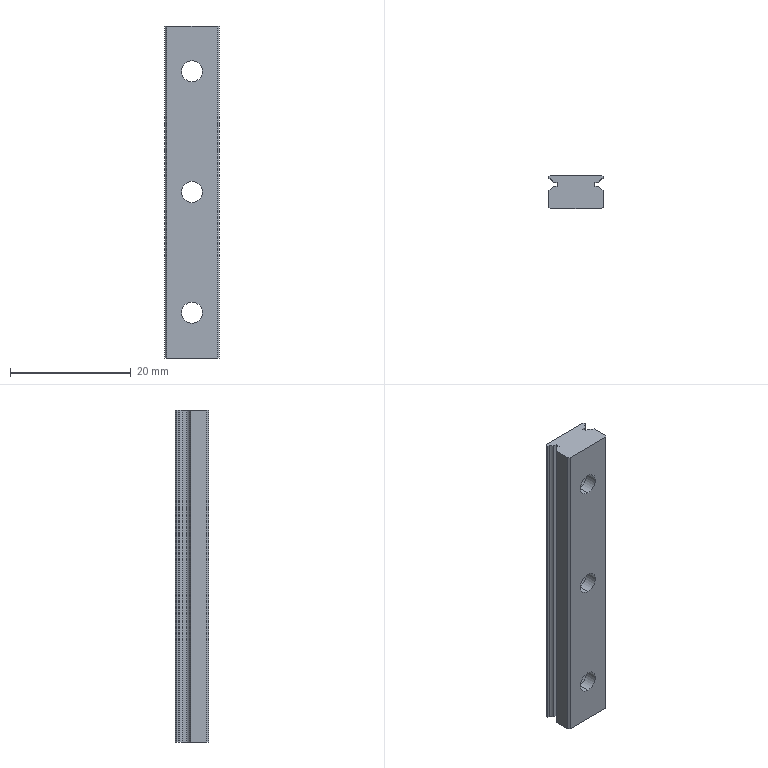Part | SolidWorks | features BaseBody 1 | 1 solid | 41 faces | box 9 x 5.5 x 55 mm | volume 2182 mm3 | plane 25 | cylinder 16 | commonest cylinder face diameters 3.5 x6 6 x6 2.2 x4
STEP:
#1=CARTESIAN_POINT('',(0.,0.,1.75));
#2=VERTEX_POINT('',#1);
#3=CARTESIAN_POINT('',(0.,0.,-1.75));
#4=VERTEX_POINT('',#3);
#5=CARTESIAN_POINT('',(0.,0.,0.));
#6=DIRECTION('',(0.,-1.,0.));
#7=DIRECTION('',(0.,0.,1.));
#8=AXIS2_PLACEMENT_3D('',#5,#6,#7);
#9=CIRCLE('',#8,1.75);
#10=EDGE_CURVE('',#2,#4,#9,.T.);
#11=ORIENTED_EDGE('',*,*,#10,.T.);
#12=CARTESIAN_POINT('',(0.,2.,-1.75));
#13=VERTEX_POINT('',#12);
#14=CARTESIAN_POINT('',(0.,0.,-1.75));
#15=DIRECTION('',(0.,1.,0.));
#16=VECTOR('',#15,1000.);
#17=LINE('',#14,#16);
#18=EDGE_CURVE('',#4,#13,#17,.T.);
#19=ORIENTED_EDGE('',*,*,#18,.T.);
#20=CARTESIAN_POINT('',(0.,2.,1.75));
#21=VERTEX_POINT('',#20);
#22=CARTESIAN_POINT('',(0.,2.,0.));
#23=DIRECTION('',(0.,-1.,0.));
#24=DIRECTION('',(0.,0.,1.));
#25=AXIS2_PLACEMENT_3D('',#22,#23,#24);
#26=CIRCLE('',#25,1.75);
#27=EDGE_CURVE('',#21,#13,#26,.T.);
#28=ORIENTED_EDGE('',*,*,#27,.F.);
#29=CARTESIAN_POINT('',(0.,0.,1.75));
#30=DIRECTION('',(0.,1.,0.));
#31=VECTOR('',#30,1000.);
#32=LINE('',#29,#31);
#33=EDGE_CURVE('',#2,#21,#32,.T.);
#34=ORIENTED_EDGE('',*,*,#33,.F.);
#35=EDGE_LOOP('',(#11,#19,#28,#34));
#36=FACE_OUTER_BOUND('',#35,.T.);
#37=CARTESIAN_POINT('',(0.,0.,0.));
#38=DIRECTION('',(0.,1.,0.));
#39=DIRECTION('',(0.,0.,1.));
#40=AXIS2_PLACEMENT_3D('',#37,#38,#39);
#41=CYLINDRICAL_SURFACE('',#40,1.75);
#42=ADVANCED_FACE('',(#36),#41,.F.);
#43=CARTESIAN_POINT('',(0.,0.,21.75));
#44=VERTEX_POINT('',#43);
#45=CARTESIAN_POINT('',(0.,0.,18.25));
#46=VERTEX_POINT('',#45);
#47=CARTESIAN_POINT('',(0.,0.,20.));
#48=DIRECTION('',(0.,-1.,0.));
#49=DIRECTION('',(0.,0.,1.));
#50=AXIS2_PLACEMENT_3D('',#47,#48,#49);
#51=CIRCLE('',#50,1.75);
#52=EDGE_CURVE('',#44,#46,#51,.T.);
#53=ORIENTED_EDGE('',*,*,#52,.T.);
#54=CARTESIAN_POINT('',(0.,2.,18.25));
#55=VERTEX_POINT('',#54);
#56=CARTESIAN_POINT('',(0.,0.,18.25));
#57=DIRECTION('',(0.,1.,0.));
#58=VECTOR('',#57,1000.);
#59=LINE('',#56,#58);
#60=EDGE_CURVE('',#46,#55,#59,.T.);
#61=ORIENTED_EDGE('',*,*,#60,.T.);
#62=CARTESIAN_POINT('',(0.,2.,21.75));
#63=VERTEX_POINT('',#62);
#64=CARTESIAN_POINT('',(0.,2.,20.));
#65=DIRECTION('',(0.,-1.,0.));
#66=DIRECTION('',(0.,0.,1.));
#67=AXIS2_PLACEMENT_3D('',#64,#65,#66);
#68=CIRCLE('',#67,1.75);
#69=EDGE_CURVE('',#63,#55,#68,.T.);
#70=ORIENTED_EDGE('',*,*,#69,.F.);
#71=CARTESIAN_POINT('',(0.,0.,21.75));
#72=DIRECTION('',(0.,1.,0.));
#73=VECTOR('',#72,1000.);
#74=LINE('',#71,#73);
#75=EDGE_CURVE('',#44,#63,#74,.T.);
#76=ORIENTED_EDGE('',*,*,#75,.F.);
#77=EDGE_LOOP('',(#53,#61,#70,#76));
#78=FACE_OUTER_BOUND('',#77,.T.);
#79=CARTESIAN_POINT('',(0.,0.,20.));
#80=DIRECTION('',(0.,1.,0.));
#81=DIRECTION('',(0.,0.,1.));
#82=AXIS2_PLACEMENT_3D('',#79,#80,#81);
#83=CYLINDRICAL_SURFACE('',#82,1.75);
#84=ADVANCED_FACE('',(#78),#83,.F.);
#85=CARTESIAN_POINT('',(0.,0.,-18.25));
#86=VERTEX_POINT('',#85);
#87=CARTESIAN_POINT('',(0.,0.,-21.75));
#88=VERTEX_POINT('',#87);
#89=CARTESIAN_POINT('',(0.,0.,-20.));
#90=DIRECTION('',(0.,-1.,0.));
#91=DIRECTION('',(0.,0.,1.));
#92=AXIS2_PLACEMENT_3D('',#89,#90,#91);
#93=CIRCLE('',#92,1.75);
#94=EDGE_CURVE('',#86,#88,#93,.T.);
#95=ORIENTED_EDGE('',*,*,#94,.T.);
#96=CARTESIAN_POINT('',(0.,2.,-21.75));
#97=VERTEX_POINT('',#96);
#98=CARTESIAN_POINT('',(0.,0.,-21.75));
#99=DIRECTION('',(0.,1.,0.));
#100=VECTOR('',#99,1000.);
#101=LINE('',#98,#100);
#102=EDGE_CURVE('',#88,#97,#101,.T.);
#103=ORIENTED_EDGE('',*,*,#102,.T.);
#104=CARTESIAN_POINT('',(0.,2.,-18.25));
#105=VERTEX_POINT('',#104);
#106=CARTESIAN_POINT('',(0.,2.,-20.));
#107=DIRECTION('',(0.,-1.,0.));
#108=DIRECTION('',(0.,0.,1.));
#109=AXIS2_PLACEMENT_3D('',#106,#107,#108);
#110=CIRCLE('',#109,1.75);
#111=EDGE_CURVE('',#105,#97,#110,.T.);
#112=ORIENTED_EDGE('',*,*,#111,.F.);
#113=CARTESIAN_POINT('',(0.,0.,-18.25));
#114=DIRECTION('',(0.,1.,0.));
#115=VECTOR('',#114,1000.);
#116=LINE('',#113,#115);
#117=EDGE_CURVE('',#86,#105,#116,.T.);
#118=ORIENTED_EDGE('',*,*,#117,.F.);
#119=EDGE_LOOP('',(#95,#103,#112,#118));
#120=FACE_OUTER_BOUND('',#119,.T.);
#121=CARTESIAN_POINT('',(0.,0.,-20.));
#122=DIRECTION('',(0.,1.,0.));
#123=DIRECTION('',(0.,0.,1.));
#124=AXIS2_PLACEMENT_3D('',#121,#122,#123);
#125=CYLINDRICAL_SURFACE('',#124,1.75);
#126=ADVANCED_FACE('',(#120),#125,.F.);
#127=CARTESIAN_POINT('',(0.,2.,-3.));
#128=VERTEX_POINT('',#127);
#129=CARTESIAN_POINT('',(0.,2.,3.));
#130=VERTEX_POINT('',#129);
#131=CARTESIAN_POINT('',(0.,2.,0.));
#132=DIRECTION('',(0.,1.,0.));
#133=DIRECTION('',(0.,0.,1.));
#134=AXIS2_PLACEMENT_3D('',#131,#132,#133);
#135=CIRCLE('',#134,3.);
#136=EDGE_CURVE('',#128,#130,#135,.T.);
#137=ORIENTED_EDGE('',*,*,#136,.F.);
#138=CARTESIAN_POINT('',(0.,5.5,-3.));
#139=VERTEX_POINT('',#138);
#140=CARTESIAN_POINT('',(0.,0.,-3.));
#141=DIRECTION('',(0.,1.,0.));
#142=VECTOR('',#141,1000.);
#143=LINE('',#140,#142);
#144=EDGE_CURVE('',#128,#139,#143,.T.);
#145=ORIENTED_EDGE('',*,*,#144,.T.);
#146=CARTESIAN_POINT('',(0.,5.5,3.));
#147=VERTEX_POINT('',#146);
#148=CARTESIAN_POINT('',(0.,5.5,0.));
#149=DIRECTION('',(0.,1.,0.));
#150=DIRECTION('',(0.,0.,1.));
#151=AXIS2_PLACEMENT_3D('',#148,#149,#150);
#152=CIRCLE('',#151,3.);
#153=EDGE_CURVE('',#139,#147,#152,.T.);
#154=ORIENTED_EDGE('',*,*,#153,.T.);
#155=CARTESIAN_POINT('',(0.,0.,3.));
#156=DIRECTION('',(0.,1.,0.));
#157=VECTOR('',#156,1000.);
#158=LINE('',#155,#157);
#159=EDGE_CURVE('',#130,#147,#158,.T.);
#160=ORIENTED_EDGE('',*,*,#159,.F.);
#161=EDGE_LOOP('',(#137,#145,#154,#160));
#162=FACE_OUTER_BOUND('',#161,.T.);
#163=CARTESIAN_POINT('',(0.,0.,0.));
#164=DIRECTION('',(0.,1.,0.));
#165=DIRECTION('',(0.,0.,1.));
#166=AXIS2_PLACEMENT_3D('',#163,#164,#165);
#167=CYLINDRICAL_SURFACE('',#166,3.);
#168=ADVANCED_FACE('',(#162),#167,.F.);
#169=CARTESIAN_POINT('',(0.,2.,17.));
#170=VERTEX_POINT('',#169);
#171=CARTESIAN_POINT('',(0.,2.,23.));
#172=VERTEX_POINT('',#171);
#173=CARTESIAN_POINT('',(0.,2.,20.));
#174=DIRECTION('',(0.,1.,0.));
#175=DIRECTION('',(0.,0.,1.));
#176=AXIS2_PLACEMENT_3D('',#173,#174,#175);
#177=CIRCLE('',#176,3.);
#178=EDGE_CURVE('',#170,#172,#177,.T.);
#179=ORIENTED_EDGE('',*,*,#178,.F.);
#180=CARTESIAN_POINT('',(0.,5.5,17.));
#181=VERTEX_POINT('',#180);
#182=CARTESIAN_POINT('',(0.,0.,17.));
#183=DIRECTION('',(0.,1.,0.));
#184=VECTOR('',#183,1000.);
#185=LINE('',#182,#184);
#186=EDGE_CURVE('',#170,#181,#185,.T.);
#187=ORIENTED_EDGE('',*,*,#186,.T.);
#188=CARTESIAN_POINT('',(0.,5.5,23.));
#189=VERTEX_POINT('',#188);
#190=CARTESIAN_POINT('',(0.,5.5,20.));
#191=DIRECTION('',(0.,1.,0.));
#192=DIRECTION('',(0.,0.,1.));
#193=AXIS2_PLACEMENT_3D('',#190,#191,#192);
#194=CIRCLE('',#193,3.);
#195=EDGE_CURVE('',#181,#189,#194,.T.);
#196=ORIENTED_EDGE('',*,*,#195,.T.);
#197=CARTESIAN_POINT('',(0.,0.,23.));
#198=DIRECTION('',(0.,1.,0.));
#199=VECTOR('',#198,1000.);
#200=LINE('',#197,#199);
#201=EDGE_CURVE('',#172,#189,#200,.T.);
#202=ORIENTED_EDGE('',*,*,#201,.F.);
#203=EDGE_LOOP('',(#179,#187,#196,#202));
#204=FACE_OUTER_BOUND('',#203,.T.);
#205=CARTESIAN_POINT('',(0.,0.,20.));
#206=DIRECTION('',(0.,1.,0.));
#207=DIRECTION('',(0.,0.,1.));
#208=AXIS2_PLACEMENT_3D('',#205,#206,#207);
#209=CYLINDRICAL_SURFACE('',#208,3.);
#210=ADVANCED_FACE('',(#204),#209,.F.);
#211=CARTESIAN_POINT('',(0.,2.,-23.));
#212=VERTEX_POINT('',#211);
#213=CARTESIAN_POINT('',(0.,2.,-17.));
#214=VERTEX_POINT('',#213);
#215=CARTESIAN_POINT('',(0.,2.,-20.));
#216=DIRECTION('',(0.,1.,0.));
#217=DIRECTION('',(0.,0.,1.));
#218=AXIS2_PLACEMENT_3D('',#215,#216,#217);
#219=CIRCLE('',#218,3.);
#220=EDGE_CURVE('',#212,#214,#219,.T.);
#221=ORIENTED_EDGE('',*,*,#220,.F.);
#222=CARTESIAN_POINT('',(0.,5.5,-23.));
#223=VERTEX_POINT('',#222);
#224=CARTESIAN_POINT('',(0.,0.,-23.));
#225=DIRECTION('',(0.,1.,0.));
#226=VECTOR('',#225,1000.);
#227=LINE('',#224,#226);
#228=EDGE_CURVE('',#212,#223,#227,.T.);
#229=ORIENTED_EDGE('',*,*,#228,.T.);
#230=CARTESIAN_POINT('',(0.,5.5,-17.));
#231=VERTEX_POINT('',#230);
#232=CARTESIAN_POINT('',(0.,5.5,-20.));
#233=DIRECTION('',(0.,1.,0.));
#234=DIRECTION('',(0.,0.,1.));
#235=AXIS2_PLACEMENT_3D('',#232,#233,#234);
#236=CIRCLE('',#235,3.);
#237=EDGE_CURVE('',#223,#231,#236,.T.);
#238=ORIENTED_EDGE('',*,*,#237,.T.);
#239=CARTESIAN_POINT('',(0.,0.,-17.));
#240=DIRECTION('',(0.,1.,0.));
#241=VECTOR('',#240,1000.);
#242=LINE('',#239,#241);
#243=EDGE_CURVE('',#214,#231,#242,.T.);
#244=ORIENTED_EDGE('',*,*,#243,.F.);
#245=EDGE_LOOP('',(#221,#229,#238,#244));
#246=FACE_OUTER_BOUND('',#245,.T.);
#247=CARTESIAN_POINT('',(0.,0.,-20.));
#248=DIRECTION('',(0.,1.,0.));
#249=DIRECTION('',(0.,0.,1.));
#250=AXIS2_PLACEMENT_3D('',#247,#248,#249);
#251=CYLINDRICAL_SURFACE('',#250,3.);
#252=ADVANCED_FACE('',(#246),#251,.F.);
#253=ORIENTED_EDGE('',*,*,#10,.F.);
#254=CARTESIAN_POINT('',(0.,0.,0.));
#255=DIRECTION('',(0.,-1.,0.));
#256=DIRECTION('',(0.,0.,1.));
#257=AXIS2_PLACEMENT_3D('',#254,#255,#256);
#258=CIRCLE('',#257,1.75);
#259=EDGE_CURVE('',#4,#2,#258,.T.);
#260=ORIENTED_EDGE('',*,*,#259,.F.);
#261=EDGE_LOOP('',(#253,#260));
#262=FACE_BOUND('',#261,.T.);
#263=ORIENTED_EDGE('',*,*,#52,.F.);
#264=CARTESIAN_POINT('',(0.,0.,20.));
#265=DIRECTION('',(0.,-1.,0.));
#266=DIRECTION('',(0.,0.,1.));
#267=AXIS2_PLACEMENT_3D('',#264,#265,#266);
#268=CIRCLE('',#267,1.75);
#269=EDGE_CURVE('',#46,#44,#268,.T.);
#270=ORIENTED_EDGE('',*,*,#269,.F.);
#271=EDGE_LOOP('',(#263,#270));
#272=FACE_BOUND('',#271,.T.);
#273=ORIENTED_EDGE('',*,*,#94,.F.);
#274=CARTESIAN_POINT('',(0.,0.,-20.));
#275=DIRECTION('',(0.,-1.,0.));
#276=DIRECTION('',(0.,0.,1.));
#277=AXIS2_PLACEMENT_3D('',#274,#275,#276);
#278=CIRCLE('',#277,1.75);
#279=EDGE_CURVE('',#88,#86,#278,.T.);
#280=ORIENTED_EDGE('',*,*,#279,.F.);
#281=EDGE_LOOP('',(#273,#280));
#282=FACE_BOUND('',#281,.T.);
#283=CARTESIAN_POINT('',(-4.2,0.,27.5));
#284=VERTEX_POINT('',#283);
#285=CARTESIAN_POINT('',(4.2,0.,27.5));
#286=VERTEX_POINT('',#285);
#287=CARTESIAN_POINT('',(-4.2,0.,27.5));
#288=DIRECTION('',(1.,0.,0.));
#289=VECTOR('',#288,1000.);
#290=LINE('',#287,#289);
#291=EDGE_CURVE('',#284,#286,#290,.T.);
#292=ORIENTED_EDGE('',*,*,#291,.F.);
#293=CARTESIAN_POINT('',(-4.2,0.,-27.5));
#294=VERTEX_POINT('',#293);
#295=CARTESIAN_POINT('',(-4.2,0.,27.5));
#296=DIRECTION('',(0.,0.,1.));
#297=VECTOR('',#296,1000.);
#298=LINE('',#295,#297);
#299=EDGE_CURVE('',#294,#284,#298,.T.);
#300=ORIENTED_EDGE('',*,*,#299,.F.);
#301=CARTESIAN_POINT('',(4.2,0.,-27.5));
#302=VERTEX_POINT('',#301);
#303=CARTESIAN_POINT('',(-4.2,0.,-27.5));
#304=DIRECTION('',(-1.,0.,0.));
#305=VECTOR('',#304,1000.);
#306=LINE('',#303,#305);
#307=EDGE_CURVE('',#302,#294,#306,.T.);
#308=ORIENTED_EDGE('',*,*,#307,.F.);
#309=CARTESIAN_POINT('',(4.2,0.,27.5));
#310=DIRECTION('',(0.,0.,-1.));
#311=VECTOR('',#310,1000.);
#312=LINE('',#309,#311);
#313=EDGE_CURVE('',#286,#302,#312,.T.);
#314=ORIENTED_EDGE('',*,*,#313,.F.);
#315=EDGE_LOOP('',(#292,#300,#308,#314));
#316=FACE_OUTER_BOUND('',#315,.T.);
#317=CARTESIAN_POINT('',(-4.2,0.,27.5));
#318=DIRECTION('',(0.,1.,0.));
#319=DIRECTION('',(0.,0.,1.));
#320=AXIS2_PLACEMENT_3D('',#317,#318,#319);
#321=PLANE('',#320);
#322=ADVANCED_FACE('',(#262,#272,#282,#316),#321,.F.);
#323=ORIENTED_EDGE('',*,*,#18,.F.);
#324=ORIENTED_EDGE('',*,*,#259,.T.);
#325=ORIENTED_EDGE('',*,*,#33,.T.);
#326=CARTESIAN_POINT('',(0.,2.,0.));
#327=DIRECTION('',(0.,-1.,0.));
#328=DIRECTION('',(0.,0.,1.));
#329=AXIS2_PLACEMENT_3D('',#326,#327,#328);
#330=CIRCLE('',#329,1.75);
#331=EDGE_CURVE('',#13,#21,#330,.T.);
#332=ORIENTED_EDGE('',*,*,#331,.F.);
#333=EDGE_LOOP('',(#323,#324,#325,#332));
#334=FACE_OUTER_BOUND('',#333,.T.);
#335=CARTESIAN_POINT('',(0.,0.,0.));
#336=DIRECTION('',(0.,1.,0.));
#337=DIRECTION('',(0.,0.,1.));
#338=AXIS2_PLACEMENT_3D('',#335,#336,#337);
#339=CYLINDRICAL_SURFACE('',#338,1.75);
#340=ADVANCED_FACE('',(#334),#339,.F.);
#341=ORIENTED_EDGE('',*,*,#60,.F.);
#342=ORIENTED_EDGE('',*,*,#269,.T.);
#343=ORIENTED_EDGE('',*,*,#75,.T.);
#344=CARTESIAN_POINT('',(0.,2.,20.));
#345=DIRECTION('',(0.,-1.,0.));
#346=DIRECTION('',(0.,0.,1.));
#347=AXIS2_PLACEMENT_3D('',#344,#345,#346);
#348=CIRCLE('',#347,1.75);
#349=EDGE_CURVE('',#55,#63,#348,.T.);
#350=ORIENTED_EDGE('',*,*,#349,.F.);
#351=EDGE_LOOP('',(#341,#342,#343,#350));
#352=FACE_OUTER_BOUND('',#351,.T.);
#353=CARTESIAN_POINT('',(0.,0.,20.));
#354=DIRECTION('',(0.,1.,0.));
#355=DIRECTION('',(0.,0.,1.));
#356=AXIS2_PLACEMENT_3D('',#353,#354,#355);
#357=CYLINDRICAL_SURFACE('',#356,1.75);
#358=ADVANCED_FACE('',(#352),#357,.F.);
#359=ORIENTED_EDGE('',*,*,#102,.F.);
#360=ORIENTED_EDGE('',*,*,#279,.T.);
#361=ORIENTED_EDGE('',*,*,#117,.T.);
#362=CARTESIAN_POINT('',(0.,2.,-20.));
#363=DIRECTION('',(0.,-1.,0.));
#364=DIRECTION('',(0.,0.,1.));
#365=AXIS2_PLACEMENT_3D('',#362,#363,#364);
#366=CIRCLE('',#365,1.75);
#367=EDGE_CURVE('',#97,#105,#366,.T.);
#368=ORIENTED_EDGE('',*,*,#367,.F.);
#369=EDGE_LOOP('',(#359,#360,#361,#368));
#370=FACE_OUTER_BOUND('',#369,.T.);
#371=CARTESIAN_POINT('',(0.,0.,-20.));
#372=DIRECTION('',(0.,1.,0.));
#373=DIRECTION('',(0.,0.,1.));
#374=AXIS2_PLACEMENT_3D('',#371,#372,#373);
#375=CYLINDRICAL_SURFACE('',#374,1.75);
#376=ADVANCED_FACE('',(#370),#375,.F.);
#377=CARTESIAN_POINT('',(4.5,0.3,27.5));
#378=VERTEX_POINT('',#377);
#379=CARTESIAN_POINT('',(4.2,0.,27.5));
#380=DIRECTION('',(0.7071,0.7071,0.));
#381=VECTOR('',#380,1000.);
#382=LINE('',#379,#381);
#383=EDGE_CURVE('',#286,#378,#382,.T.);
#384=ORIENTED_EDGE('',*,*,#383,.F.);
#385=ORIENTED_EDGE('',*,*,#313,.T.);
#386=CARTESIAN_POINT('',(4.5,0.3,-27.5));
#387=VERTEX_POINT('',#386);
#388=CARTESIAN_POINT('',(4.2,0.,-27.5));
#389=DIRECTION('',(-0.7071,-0.7071,0.));
#390=VECTOR('',#389,1000.);
#391=LINE('',#388,#390);
#392=EDGE_CURVE('',#387,#302,#391,.T.);
#393=ORIENTED_EDGE('',*,*,#392,.F.);
#394=CARTESIAN_POINT('',(4.5,0.3,27.5));
#395=DIRECTION('',(0.,0.,-1.));
#396=VECTOR('',#395,1000.);
#397=LINE('',#394,#396);
#398=EDGE_CURVE('',#378,#387,#397,.T.);
#399=ORIENTED_EDGE('',*,*,#398,.F.);
#400=EDGE_LOOP('',(#384,#385,#393,#399));
#401=FACE_OUTER_BOUND('',#400,.T.);
#402=CARTESIAN_POINT('',(4.2,0.,27.5));
#403=DIRECTION('',(-0.7071,0.7071,0.));
#404=DIRECTION('',(-0.7071,-0.7071,0.));
#405=AXIS2_PLACEMENT_3D('',#402,#403,#404);
#406=PLANE('',#405);
#407=ADVANCED_FACE('',(#401),#406,.F.);
#408=CARTESIAN_POINT('',(4.222,4.883,27.5));
#409=VERTEX_POINT('',#408);
#410=CARTESIAN_POINT('',(4.5,5.043,27.5));
#411=VERTEX_POINT('',#410);
#412=CARTESIAN_POINT('',(4.222,4.883,27.5));
#413=DIRECTION('',(0.8661,0.5,0.));
#414=VECTOR('',#413,1000.);
#415=LINE('',#412,#414);
#416=EDGE_CURVE('',#409,#411,#415,.T.);
#417=ORIENTED_EDGE('',*,*,#416,.T.);
#418=CARTESIAN_POINT('',(4.5,5.3,27.5));
#419=VERTEX_POINT('',#418);
#420=CARTESIAN_POINT('',(4.5,5.043,27.5));
#421=DIRECTION('',(0.,1.,0.));
#422=VECTOR('',#421,1000.);
#423=LINE('',#420,#422);
#424=EDGE_CURVE('',#411,#419,#423,.T.);
#425=ORIENTED_EDGE('',*,*,#424,.T.);
#426=CARTESIAN_POINT('',(4.3,5.5,27.5));
#427=VERTEX_POINT('',#426);
#428=CARTESIAN_POINT('',(4.5,5.3,27.5));
#429=DIRECTION('',(-0.7071,0.7071,0.));
#430=VECTOR('',#429,1000.);
#431=LINE('',#428,#430);
#432=EDGE_CURVE('',#419,#427,#431,.T.);
#433=ORIENTED_EDGE('',*,*,#432,.T.);
#434=CARTESIAN_POINT('',(-4.3,5.5,27.5));
#435=VERTEX_POINT('',#434);
#436=CARTESIAN_POINT('',(-4.771,5.5,27.5));
#437=DIRECTION('',(-1.,0.,0.));
#438=VECTOR('',#437,1000.);
#439=LINE('',#436,#438);
#440=EDGE_CURVE('',#427,#435,#439,.T.);
#441=ORIENTED_EDGE('',*,*,#440,.T.);
#442=CARTESIAN_POINT('',(-4.5,5.3,27.5));
#443=VERTEX_POINT('',#442);
#444=CARTESIAN_POINT('',(-4.3,5.5,27.5));
#445=DIRECTION('',(-0.7071,-0.7071,0.));
#446=VECTOR('',#445,1000.);
#447=LINE('',#444,#446);
#448=EDGE_CURVE('',#435,#443,#447,.T.);
#449=ORIENTED_EDGE('',*,*,#448,.T.);
#450=CARTESIAN_POINT('',(-4.5,5.043,27.5));
#451=VERTEX_POINT('',#450);
#452=CARTESIAN_POINT('',(-4.5,5.3,27.5));
#453=DIRECTION('',(0.,-1.,0.));
#454=VECTOR('',#453,1000.);
#455=LINE('',#452,#454);
#456=EDGE_CURVE('',#443,#451,#455,.T.);
#457=ORIENTED_EDGE('',*,*,#456,.T.);
#458=CARTESIAN_POINT('',(-4.222,4.883,27.5));
#459=VERTEX_POINT('',#458);
#460=CARTESIAN_POINT('',(-4.5,5.043,27.5));
#461=DIRECTION('',(0.8661,-0.5,0.));
#462=VECTOR('',#461,1000.);
#463=LINE('',#460,#462);
#464=EDGE_CURVE('',#451,#459,#463,.T.);
#465=ORIENTED_EDGE('',*,*,#464,.T.);
#466=CARTESIAN_POINT('',(-3.755,4.35,27.5));
#467=VERTEX_POINT('',#466);
#468=CARTESIAN_POINT('',(-4.771,3.93,27.5));
#469=DIRECTION('',(0.,0.,-1.));
#470=DIRECTION('',(1.,0.,0.));
#471=AXIS2_PLACEMENT_3D('',#468,#469,#470);
#472=CIRCLE('',#471,1.1);
#473=EDGE_CURVE('',#459,#467,#472,.T.);
#474=ORIENTED_EDGE('',*,*,#473,.T.);
#475=CARTESIAN_POINT('',(-3.1,4.35,27.5));
#476=VERTEX_POINT('',#475);
#477=CARTESIAN_POINT('',(-3.755,4.35,27.5));
#478=DIRECTION('',(1.,0.,0.));
#479=VECTOR('',#478,1000.);
#480=LINE('',#477,#479);
#481=EDGE_CURVE('',#467,#476,#480,.T.);
#482=ORIENTED_EDGE('',*,*,#481,.T.);
#483=CARTESIAN_POINT('',(-3.1,3.65,27.5));
#484=VERTEX_POINT('',#483);
#485=CARTESIAN_POINT('',(-3.1,4.35,27.5));
#486=DIRECTION('',(0.,-1.,0.));
#487=VECTOR('',#486,1000.);
#488=LINE('',#485,#487);
#489=EDGE_CURVE('',#476,#484,#488,.T.);
#490=ORIENTED_EDGE('',*,*,#489,.T.);
#491=CARTESIAN_POINT('',(-3.755,3.65,27.5));
#492=VERTEX_POINT('',#491);
#493=CARTESIAN_POINT('',(-3.1,3.65,27.5));
#494=DIRECTION('',(-1.,0.,0.));
#495=VECTOR('',#494,1000.);
#496=LINE('',#493,#495);
#497=EDGE_CURVE('',#484,#492,#496,.T.);
#498=ORIENTED_EDGE('',*,*,#497,.T.);
#499=CARTESIAN_POINT('',(-4.222,3.117,27.5));
#500=VERTEX_POINT('',#499);
#501=CARTESIAN_POINT('',(-4.772,4.07,27.5));
#502=DIRECTION('',(0.,0.,-1.));
#503=DIRECTION('',(1.,0.,0.));
#504=AXIS2_PLACEMENT_3D('',#501,#502,#503);
#505=CIRCLE('',#504,1.1);
#506=EDGE_CURVE('',#492,#500,#505,.T.);
#507=ORIENTED_EDGE('',*,*,#506,.T.);
#508=CARTESIAN_POINT('',(-4.5,2.957,27.5));
#509=VERTEX_POINT('',#508);
#510=CARTESIAN_POINT('',(-4.222,3.117,27.5));
#511=DIRECTION('',(-0.8661,-0.5,0.));
#512=VECTOR('',#511,1000.);
#513=LINE('',#510,#512);
#514=EDGE_CURVE('',#500,#509,#513,.T.);
#515=ORIENTED_EDGE('',*,*,#514,.T.);
#516=CARTESIAN_POINT('',(-4.5,0.3,27.5));
#517=VERTEX_POINT('',#516);
#518=CARTESIAN_POINT('',(-4.5,3.93,27.5));
#519=DIRECTION('',(0.,-1.,0.));
#520=VECTOR('',#519,1000.);
#521=LINE('',#518,#520);
#522=EDGE_CURVE('',#509,#517,#521,.T.);
#523=ORIENTED_EDGE('',*,*,#522,.T.);
#524=CARTESIAN_POINT('',(-4.5,0.3,27.5));
#525=DIRECTION('',(0.7071,-0.7071,0.));
#526=VECTOR('',#525,1000.);
#527=LINE('',#524,#526);
#528=EDGE_CURVE('',#517,#284,#527,.T.);
#529=ORIENTED_EDGE('',*,*,#528,.T.);
#530=ORIENTED_EDGE('',*,*,#291,.T.);
#531=ORIENTED_EDGE('',*,*,#383,.T.);
#532=CARTESIAN_POINT('',(4.5,2.957,27.5));
#533=VERTEX_POINT('',#532);
#534=CARTESIAN_POINT('',(4.5,3.93,27.5));
#535=DIRECTION('',(0.,1.,0.));
#536=VECTOR('',#535,1000.);
#537=LINE('',#534,#536);
#538=EDGE_CURVE('',#378,#533,#537,.T.);
#539=ORIENTED_EDGE('',*,*,#538,.T.);
#540=CARTESIAN_POINT('',(4.222,3.117,27.5));
#541=VERTEX_POINT('',#540);
#542=CARTESIAN_POINT('',(4.5,2.957,27.5));
#543=DIRECTION('',(-0.8661,0.5,0.));
#544=VECTOR('',#543,1000.);
#545=LINE('',#542,#544);
#546=EDGE_CURVE('',#533,#541,#545,.T.);
#547=ORIENTED_EDGE('',*,*,#546,.T.);
#548=CARTESIAN_POINT('',(3.755,3.65,27.5));
#549=VERTEX_POINT('',#548);
#550=CARTESIAN_POINT('',(4.772,4.07,27.5));
#551=DIRECTION('',(0.,0.,-1.));
#552=DIRECTION('',(1.,0.,0.));
#553=AXIS2_PLACEMENT_3D('',#550,#551,#552);
#554=CIRCLE('',#553,1.1);
#555=EDGE_CURVE('',#541,#549,#554,.T.);
#556=ORIENTED_EDGE('',*,*,#555,.T.);
#557=CARTESIAN_POINT('',(3.1,3.65,27.5));
#558=VERTEX_POINT('',#557);
#559=CARTESIAN_POINT('',(3.755,3.65,27.5));
#560=DIRECTION('',(-1.,0.,0.));
#561=VECTOR('',#560,1000.);
#562=LINE('',#559,#561);
#563=EDGE_CURVE('',#549,#558,#562,.T.);
#564=ORIENTED_EDGE('',*,*,#563,.T.);
#565=CARTESIAN_POINT('',(3.1,4.35,27.5));
#566=VERTEX_POINT('',#565);
#567=CARTESIAN_POINT('',(3.1,3.65,27.5));
#568=DIRECTION('',(0.,1.,0.));
#569=VECTOR('',#568,1000.);
#570=LINE('',#567,#569);
#571=EDGE_CURVE('',#558,#566,#570,.T.);
#572=ORIENTED_EDGE('',*,*,#571,.T.);
#573=CARTESIAN_POINT('',(3.755,4.35,27.5));
#574=VERTEX_POINT('',#573);
#575=CARTESIAN_POINT('',(3.1,4.35,27.5));
#576=DIRECTION('',(1.,0.,0.));
#577=VECTOR('',#576,1000.);
#578=LINE('',#575,#577);
#579=EDGE_CURVE('',#566,#574,#578,.T.);
#580=ORIENTED_EDGE('',*,*,#579,.T.);
#581=CARTESIAN_POINT('',(4.771,3.93,27.5));
#582=DIRECTION('',(0.,0.,-1.));
#583=DIRECTION('',(1.,0.,0.));
#584=AXIS2_PLACEMENT_3D('',#581,#582,#583);
#585=CIRCLE('',#584,1.1);
#586=EDGE_CURVE('',#574,#409,#585,.T.);
#587=ORIENTED_EDGE('',*,*,#586,.T.);
#588=EDGE_LOOP('',(#417,#425,#433,#441,#449,#457,#465,#474,#482,#490,#498,#507,#515,#523,#529,#530,#531,#539,#547,#556,#564,#572,#580,#587));
#589=FACE_OUTER_BOUND('',#588,.T.);
#590=CARTESIAN_POINT('',(-4.771,3.93,27.5));
#591=DIRECTION('',(0.,0.,1.));
#592=DIRECTION('',(1.,0.,0.));
#593=AXIS2_PLACEMENT_3D('',#590,#591,#592);
#594=PLANE('',#593);
#595=ADVANCED_FACE('',(#589),#594,.T.);
#596=ORIENTED_EDGE('',*,*,#528,.F.);
#597=CARTESIAN_POINT('',(-4.5,0.3,-27.5));
#598=VERTEX_POINT('',#597);
#599=CARTESIAN_POINT('',(-4.5,0.3,27.5));
#600=DIRECTION('',(0.,0.,1.));
#601=VECTOR('',#600,1000.);
#602=LINE('',#599,#601);
#603=EDGE_CURVE('',#598,#517,#602,.T.);
#604=ORIENTED_EDGE('',*,*,#603,.F.);
#605=CARTESIAN_POINT('',(-4.5,0.3,-27.5));
#606=DIRECTION('',(-0.7071,0.7071,0.));
#607=VECTOR('',#606,1000.);
#608=LINE('',#605,#607);
#609=EDGE_CURVE('',#294,#598,#608,.T.);
#610=ORIENTED_EDGE('',*,*,#609,.F.);
#611=ORIENTED_EDGE('',*,*,#299,.T.);
#612=EDGE_LOOP('',(#596,#604,#610,#611));
#613=FACE_OUTER_BOUND('',#612,.T.);
#614=CARTESIAN_POINT('',(-4.5,0.3,27.5));
#615=DIRECTION('',(0.7071,0.7071,0.));
#616=DIRECTION('',(-0.7071,0.7071,0.));
#617=AXIS2_PLACEMENT_3D('',#614,#615,#616);
#618=PLANE('',#617);
#619=ADVANCED_FACE('',(#613),#618,.F.);
#620=CARTESIAN_POINT('',(4.3,5.5,-27.5));
#621=VERTEX_POINT('',#620);
#622=CARTESIAN_POINT('',(4.5,5.3,-27.5));
#623=VERTEX_POINT('',#622);
#624=CARTESIAN_POINT('',(4.5,5.3,-27.5));
#625=DIRECTION('',(0.7071,-0.7071,0.));
#626=VECTOR('',#625,1000.);
#627=LINE('',#624,#626);
#628=EDGE_CURVE('',#621,#623,#627,.T.);
#629=ORIENTED_EDGE('',*,*,#628,.T.);
#630=CARTESIAN_POINT('',(4.5,5.043,-27.5));
#631=VERTEX_POINT('',#630);
#632=CARTESIAN_POINT('',(4.5,5.043,-27.5));
#633=DIRECTION('',(0.,-1.,0.));
#634=VECTOR('',#633,1000.);
#635=LINE('',#632,#634);
#636=EDGE_CURVE('',#623,#631,#635,.T.);
#637=ORIENTED_EDGE('',*,*,#636,.T.);
#638=CARTESIAN_POINT('',(4.222,4.883,-27.5));
#639=VERTEX_POINT('',#638);
#640=CARTESIAN_POINT('',(4.222,4.883,-27.5));
#641=DIRECTION('',(-0.8661,-0.5,0.));
#642=VECTOR('',#641,1000.);
#643=LINE('',#640,#642);
#644=EDGE_CURVE('',#631,#639,#643,.T.);
#645=ORIENTED_EDGE('',*,*,#644,.T.);
#646=CARTESIAN_POINT('',(3.755,4.35,-27.5));
#647=VERTEX_POINT('',#646);
#648=CARTESIAN_POINT('',(4.771,3.93,-27.5));
#649=DIRECTION('',(0.,0.,1.));
#650=DIRECTION('',(1.,0.,0.));
#651=AXIS2_PLACEMENT_3D('',#648,#649,#650);
#652=CIRCLE('',#651,1.1);
#653=EDGE_CURVE('',#639,#647,#652,.T.);
#654=ORIENTED_EDGE('',*,*,#653,.T.);
#655=CARTESIAN_POINT('',(3.1,4.35,-27.5));
#656=VERTEX_POINT('',#655);
#657=CARTESIAN_POINT('',(3.1,4.35,-27.5));
#658=DIRECTION('',(-1.,0.,0.));
#659=VECTOR('',#658,1000.);
#660=LINE('',#657,#659);
#661=EDGE_CURVE('',#647,#656,#660,.T.);
#662=ORIENTED_EDGE('',*,*,#661,.T.);
#663=CARTESIAN_POINT('',(3.1,3.65,-27.5));
#664=VERTEX_POINT('',#663);
#665=CARTESIAN_POINT('',(3.1,3.65,-27.5));
#666=DIRECTION('',(0.,-1.,0.));
#667=VECTOR('',#666,1000.);
#668=LINE('',#665,#667);
#669=EDGE_CURVE('',#656,#664,#668,.T.);
#670=ORIENTED_EDGE('',*,*,#669,.T.);
#671=CARTESIAN_POINT('',(3.755,3.65,-27.5));
#672=VERTEX_POINT('',#671);
#673=CARTESIAN_POINT('',(3.755,3.65,-27.5));
#674=DIRECTION('',(1.,0.,0.));
#675=VECTOR('',#674,1000.);
#676=LINE('',#673,#675);
#677=EDGE_CURVE('',#664,#672,#676,.T.);
#678=ORIENTED_EDGE('',*,*,#677,.T.);
#679=CARTESIAN_POINT('',(4.222,3.117,-27.5));
#680=VERTEX_POINT('',#679);
#681=CARTESIAN_POINT('',(4.772,4.07,-27.5));
#682=DIRECTION('',(0.,0.,1.));
#683=DIRECTION('',(1.,0.,0.));
#684=AXIS2_PLACEMENT_3D('',#681,#682,#683);
#685=CIRCLE('',#684,1.1);
#686=EDGE_CURVE('',#672,#680,#685,.T.);
#687=ORIENTED_EDGE('',*,*,#686,.T.);
#688=CARTESIAN_POINT('',(4.5,2.957,-27.5));
#689=VERTEX_POINT('',#688);
#690=CARTESIAN_POINT('',(4.5,2.957,-27.5));
#691=DIRECTION('',(0.8661,-0.5,0.));
#692=VECTOR('',#691,1000.);
#693=LINE('',#690,#692);
#694=EDGE_CURVE('',#680,#689,#693,.T.);
#695=ORIENTED_EDGE('',*,*,#694,.T.);
#696=CARTESIAN_POINT('',(4.5,3.93,-27.5));
#697=DIRECTION('',(0.,1.,0.));
#698=VECTOR('',#697,1000.);
#699=LINE('',#696,#698);
#700=EDGE_CURVE('',#387,#689,#699,.T.);
#701=ORIENTED_EDGE('',*,*,#700,.F.);
#702=ORIENTED_EDGE('',*,*,#392,.T.);
#703=ORIENTED_EDGE('',*,*,#307,.T.);
#704=ORIENTED_EDGE('',*,*,#609,.T.);
#705=CARTESIAN_POINT('',(-4.5,2.957,-27.5));
#706=VERTEX_POINT('',#705);
#707=CARTESIAN_POINT('',(-4.5,3.93,-27.5));
#708=DIRECTION('',(0.,-1.,0.));
#709=VECTOR('',#708,1000.);
#710=LINE('',#707,#709);
#711=EDGE_CURVE('',#706,#598,#710,.T.);
#712=ORIENTED_EDGE('',*,*,#711,.F.);
#713=CARTESIAN_POINT('',(-4.222,3.117,-27.5));
#714=VERTEX_POINT('',#713);
#715=CARTESIAN_POINT('',(-4.222,3.117,-27.5));
#716=DIRECTION('',(0.8661,0.5,0.));
#717=VECTOR('',#716,1000.);
#718=LINE('',#715,#717);
#719=EDGE_CURVE('',#706,#714,#718,.T.);
#720=ORIENTED_EDGE('',*,*,#719,.T.);
#721=CARTESIAN_POINT('',(-3.755,3.65,-27.5));
#722=VERTEX_POINT('',#721);
#723=CARTESIAN_POINT('',(-4.772,4.07,-27.5));
#724=DIRECTION('',(0.,0.,1.));
#725=DIRECTION('',(1.,0.,0.));
#726=AXIS2_PLACEMENT_3D('',#723,#724,#725);
#727=CIRCLE('',#726,1.1);
#728=EDGE_CURVE('',#714,#722,#727,.T.);
#729=ORIENTED_EDGE('',*,*,#728,.T.);
#730=CARTESIAN_POINT('',(-3.1,3.65,-27.5));
#731=VERTEX_POINT('',#730);
#732=CARTESIAN_POINT('',(-3.1,3.65,-27.5));
#733=DIRECTION('',(1.,0.,0.));
#734=VECTOR('',#733,1000.);
#735=LINE('',#732,#734);
#736=EDGE_CURVE('',#722,#731,#735,.T.);
#737=ORIENTED_EDGE('',*,*,#736,.T.);
#738=CARTESIAN_POINT('',(-3.1,4.35,-27.5));
#739=VERTEX_POINT('',#738);
#740=CARTESIAN_POINT('',(-3.1,4.35,-27.5));
#741=DIRECTION('',(0.,1.,0.));
#742=VECTOR('',#741,1000.);
#743=LINE('',#740,#742);
#744=EDGE_CURVE('',#731,#739,#743,.T.);
#745=ORIENTED_EDGE('',*,*,#744,.T.);
#746=CARTESIAN_POINT('',(-3.755,4.35,-27.5));
#747=VERTEX_POINT('',#746);
#748=CARTESIAN_POINT('',(-3.755,4.35,-27.5));
#749=DIRECTION('',(-1.,0.,0.));
#750=VECTOR('',#749,1000.);
#751=LINE('',#748,#750);
#752=EDGE_CURVE('',#739,#747,#751,.T.);
#753=ORIENTED_EDGE('',*,*,#752,.T.);
#754=CARTESIAN_POINT('',(-4.222,4.883,-27.5));
#755=VERTEX_POINT('',#754);
#756=CARTESIAN_POINT('',(-4.771,3.93,-27.5));
#757=DIRECTION('',(0.,0.,1.));
#758=DIRECTION('',(1.,0.,0.));
#759=AXIS2_PLACEMENT_3D('',#756,#757,#758);
#760=CIRCLE('',#759,1.1);
#761=EDGE_CURVE('',#747,#755,#760,.T.);
#762=ORIENTED_EDGE('',*,*,#761,.T.);
#763=CARTESIAN_POINT('',(-4.5,5.043,-27.5));
#764=VERTEX_POINT('',#763);
#765=CARTESIAN_POINT('',(-4.5,5.043,-27.5));
#766=DIRECTION('',(-0.8661,0.5,0.));
#767=VECTOR('',#766,1000.);
#768=LINE('',#765,#767);
#769=EDGE_CURVE('',#755,#764,#768,.T.);
#770=ORIENTED_EDGE('',*,*,#769,.T.);
#771=CARTESIAN_POINT('',(-4.5,5.3,-27.5));
#772=VERTEX_POINT('',#771);
#773=CARTESIAN_POINT('',(-4.5,5.3,-27.5));
#774=DIRECTION('',(0.,1.,0.));
#775=VECTOR('',#774,1000.);
#776=LINE('',#773,#775);
#777=EDGE_CURVE('',#764,#772,#776,.T.);
#778=ORIENTED_EDGE('',*,*,#777,.T.);
#779=CARTESIAN_POINT('',(-4.3,5.5,-27.5));
#780=VERTEX_POINT('',#779);
#781=CARTESIAN_POINT('',(-4.3,5.5,-27.5));
#782=DIRECTION('',(0.7071,0.7071,0.));
#783=VECTOR('',#782,1000.);
#784=LINE('',#781,#783);
#785=EDGE_CURVE('',#772,#780,#784,.T.);
#786=ORIENTED_EDGE('',*,*,#785,.T.);
#787=CARTESIAN_POINT('',(-4.771,5.5,-27.5));
#788=DIRECTION('',(-1.,0.,0.));
#789=VECTOR('',#788,1000.);
#790=LINE('',#787,#789);
#791=EDGE_CURVE('',#621,#780,#790,.T.);
#792=ORIENTED_EDGE('',*,*,#791,.F.);
#793=EDGE_LOOP('',(#629,#637,#645,#654,#662,#670,#678,#687,#695,#701,#702,#703,#704,#712,#720,#729,#737,#745,#753,#762,#770,#778,#786,#792));
#794=FACE_OUTER_BOUND('',#793,.T.);
#795=CARTESIAN_POINT('',(-4.771,3.93,-27.5));
#796=DIRECTION('',(0.,0.,1.));
#797=DIRECTION('',(1.,0.,0.));
#798=AXIS2_PLACEMENT_3D('',#795,#796,#797);
#799=PLANE('',#798);
#800=ADVANCED_FACE('',(#794),#799,.F.);
#801=ORIENTED_EDGE('',*,*,#27,.T.);
#802=ORIENTED_EDGE('',*,*,#331,.T.);
#803=EDGE_LOOP('',(#801,#802));
#804=FACE_BOUND('',#803,.T.);
#805=CARTESIAN_POINT('',(0.,2.,0.));
#806=DIRECTION('',(0.,1.,0.));
#807=DIRECTION('',(0.,0.,1.));
#808=AXIS2_PLACEMENT_3D('',#805,#806,#807);
#809=CIRCLE('',#808,3.);
#810=EDGE_CURVE('',#130,#128,#809,.T.);
#811=ORIENTED_EDGE('',*,*,#810,.T.);
#812=ORIENTED_EDGE('',*,*,#136,.T.);
#813=EDGE_LOOP('',(#811,#812));
#814=FACE_OUTER_BOUND('',#813,.T.);
#815=CARTESIAN_POINT('',(0.,2.,-3.));
#816=DIRECTION('',(0.,1.,0.));
#817=DIRECTION('',(0.,0.,1.));
#818=AXIS2_PLACEMENT_3D('',#815,#816,#817);
#819=PLANE('',#818);
#820=ADVANCED_FACE('',(#804,#814),#819,.T.);
#821=ORIENTED_EDGE('',*,*,#69,.T.);
#822=ORIENTED_EDGE('',*,*,#349,.T.);
#823=EDGE_LOOP('',(#821,#822));
#824=FACE_BOUND('',#823,.T.);
#825=CARTESIAN_POINT('',(0.,2.,20.));
#826=DIRECTION('',(0.,1.,0.));
#827=DIRECTION('',(0.,0.,1.));
#828=AXIS2_PLACEMENT_3D('',#825,#826,#827);
#829=CIRCLE('',#828,3.);
#830=EDGE_CURVE('',#172,#170,#829,.T.);
#831=ORIENTED_EDGE('',*,*,#830,.T.);
#832=ORIENTED_EDGE('',*,*,#178,.T.);
#833=EDGE_LOOP('',(#831,#832));
#834=FACE_OUTER_BOUND('',#833,.T.);
#835=CARTESIAN_POINT('',(0.,2.,17.));
#836=DIRECTION('',(0.,1.,0.));
#837=DIRECTION('',(0.,0.,1.));
#838=AXIS2_PLACEMENT_3D('',#835,#836,#837);
#839=PLANE('',#838);
#840=ADVANCED_FACE('',(#824,#834),#839,.T.);
#841=ORIENTED_EDGE('',*,*,#111,.T.);
#842=ORIENTED_EDGE('',*,*,#367,.T.);
#843=EDGE_LOOP('',(#841,#842));
#844=FACE_BOUND('',#843,.T.);
#845=CARTESIAN_POINT('',(0.,2.,-20.));
#846=DIRECTION('',(0.,1.,0.));
#847=DIRECTION('',(0.,0.,1.));
#848=AXIS2_PLACEMENT_3D('',#845,#846,#847);
#849=CIRCLE('',#848,3.);
#850=EDGE_CURVE('',#214,#212,#849,.T.);
#851=ORIENTED_EDGE('',*,*,#850,.T.);
#852=ORIENTED_EDGE('',*,*,#220,.T.);
#853=EDGE_LOOP('',(#851,#852));
#854=FACE_OUTER_BOUND('',#853,.T.);
#855=CARTESIAN_POINT('',(0.,2.,-23.));
#856=DIRECTION('',(0.,1.,0.));
#857=DIRECTION('',(0.,0.,1.));
#858=AXIS2_PLACEMENT_3D('',#855,#856,#857);
#859=PLANE('',#858);
#860=ADVANCED_FACE('',(#844,#854),#859,.T.);
#861=ORIENTED_EDGE('',*,*,#538,.F.);
#862=ORIENTED_EDGE('',*,*,#398,.T.);
#863=ORIENTED_EDGE('',*,*,#700,.T.);
#864=CARTESIAN_POINT('',(4.5,2.957,27.5));
#865=DIRECTION('',(0.,0.,-1.));
#866=VECTOR('',#865,1000.);
#867=LINE('',#864,#866);
#868=EDGE_CURVE('',#533,#689,#867,.T.);
#869=ORIENTED_EDGE('',*,*,#868,.F.);
#870=EDGE_LOOP('',(#861,#862,#863,#869));
#871=FACE_OUTER_BOUND('',#870,.T.);
#872=CARTESIAN_POINT('',(4.5,0.3,27.5));
#873=DIRECTION('',(-1.,0.,0.));
#874=DIRECTION('',(0.,0.,1.));
#875=AXIS2_PLACEMENT_3D('',#872,#873,#874);
#876=PLANE('',#875);
#877=ADVANCED_FACE('',(#871),#876,.F.);
#878=ORIENTED_EDGE('',*,*,#522,.F.);
#879=CARTESIAN_POINT('',(-4.5,2.957,27.5));
#880=DIRECTION('',(0.,0.,1.));
#881=VECTOR('',#880,1000.);
#882=LINE('',#879,#881);
#883=EDGE_CURVE('',#706,#509,#882,.T.);
#884=ORIENTED_EDGE('',*,*,#883,.F.);
#885=ORIENTED_EDGE('',*,*,#711,.T.);
#886=ORIENTED_EDGE('',*,*,#603,.T.);
#887=EDGE_LOOP('',(#878,#884,#885,#886));
#888=FACE_OUTER_BOUND('',#887,.T.);
#889=CARTESIAN_POINT('',(-4.5,2.957,27.5));
#890=DIRECTION('',(1.,0.,0.));
#891=DIRECTION('',(0.,0.,-1.));
#892=AXIS2_PLACEMENT_3D('',#889,#890,#891);
#893=PLANE('',#892);
#894=ADVANCED_FACE('',(#888),#893,.F.);
#895=CARTESIAN_POINT('',(0.,5.5,0.));
#896=DIRECTION('',(0.,1.,0.));
#897=DIRECTION('',(0.,0.,1.));
#898=AXIS2_PLACEMENT_3D('',#895,#896,#897);
#899=CIRCLE('',#898,3.);
#900=EDGE_CURVE('',#147,#139,#899,.T.);
#901=ORIENTED_EDGE('',*,*,#900,.F.);
#902=ORIENTED_EDGE('',*,*,#153,.F.);
#903=EDGE_LOOP('',(#901,#902));
#904=FACE_BOUND('',#903,.T.);
#905=CARTESIAN_POINT('',(0.,5.5,20.));
#906=DIRECTION('',(0.,1.,0.));
#907=DIRECTION('',(0.,0.,1.));
#908=AXIS2_PLACEMENT_3D('',#905,#906,#907);
#909=CIRCLE('',#908,3.);
#910=EDGE_CURVE('',#189,#181,#909,.T.);
#911=ORIENTED_EDGE('',*,*,#910,.F.);
#912=ORIENTED_EDGE('',*,*,#195,.F.);
#913=EDGE_LOOP('',(#911,#912));
#914=FACE_BOUND('',#913,.T.);
#915=CARTESIAN_POINT('',(0.,5.5,-20.));
#916=DIRECTION('',(0.,1.,0.));
#917=DIRECTION('',(0.,0.,1.));
#918=AXIS2_PLACEMENT_3D('',#915,#916,#917);
#919=CIRCLE('',#918,3.);
#920=EDGE_CURVE('',#231,#223,#919,.T.);
#921=ORIENTED_EDGE('',*,*,#920,.F.);
#922=ORIENTED_EDGE('',*,*,#237,.F.);
#923=EDGE_LOOP('',(#921,#922));
#924=FACE_BOUND('',#923,.T.);
#925=ORIENTED_EDGE('',*,*,#440,.F.);
#926=CARTESIAN_POINT('',(4.3,5.5,27.5));
#927=DIRECTION('',(0.,0.,1.));
#928=VECTOR('',#927,1000.);
#929=LINE('',#926,#928);
#930=EDGE_CURVE('',#621,#427,#929,.T.);
#931=ORIENTED_EDGE('',*,*,#930,.F.);
#932=ORIENTED_EDGE('',*,*,#791,.T.);
#933=CARTESIAN_POINT('',(-4.3,5.5,27.5));
#934=DIRECTION('',(0.,0.,-1.));
#935=VECTOR('',#934,1000.);
#936=LINE('',#933,#935);
#937=EDGE_CURVE('',#435,#780,#936,.T.);
#938=ORIENTED_EDGE('',*,*,#937,.F.);
#939=EDGE_LOOP('',(#925,#931,#932,#938));
#940=FACE_OUTER_BOUND('',#939,.T.);
#941=CARTESIAN_POINT('',(4.3,5.5,27.5));
#942=DIRECTION('',(0.,-1.,0.));
#943=DIRECTION('',(0.,0.,-1.));
#944=AXIS2_PLACEMENT_3D('',#941,#942,#943);
#945=PLANE('',#944);
#946=ADVANCED_FACE('',(#904,#914,#924,#940),#945,.F.);
#947=ORIENTED_EDGE('',*,*,#144,.F.);
#948=ORIENTED_EDGE('',*,*,#810,.F.);
#949=ORIENTED_EDGE('',*,*,#159,.T.);
#950=ORIENTED_EDGE('',*,*,#900,.T.);
#951=EDGE_LOOP('',(#947,#948,#949,#950));
#952=FACE_OUTER_BOUND('',#951,.T.);
#953=CARTESIAN_POINT('',(0.,0.,0.));
#954=DIRECTION('',(0.,1.,0.));
#955=DIRECTION('',(0.,0.,1.));
#956=AXIS2_PLACEMENT_3D('',#953,#954,#955);
#957=CYLINDRICAL_SURFACE('',#956,3.);
#958=ADVANCED_FACE('',(#952),#957,.F.);
#959=ORIENTED_EDGE('',*,*,#186,.F.);
#960=ORIENTED_EDGE('',*,*,#830,.F.);
#961=ORIENTED_EDGE('',*,*,#201,.T.);
#962=ORIENTED_EDGE('',*,*,#910,.T.);
#963=EDGE_LOOP('',(#959,#960,#961,#962));
#964=FACE_OUTER_BOUND('',#963,.T.);
#965=CARTESIAN_POINT('',(0.,0.,20.));
#966=DIRECTION('',(0.,1.,0.));
#967=DIRECTION('',(0.,0.,1.));
#968=AXIS2_PLACEMENT_3D('',#965,#966,#967);
#969=CYLINDRICAL_SURFACE('',#968,3.);
#970=ADVANCED_FACE('',(#964),#969,.F.);
#971=ORIENTED_EDGE('',*,*,#228,.F.);
#972=ORIENTED_EDGE('',*,*,#850,.F.);
#973=ORIENTED_EDGE('',*,*,#243,.T.);
#974=ORIENTED_EDGE('',*,*,#920,.T.);
#975=EDGE_LOOP('',(#971,#972,#973,#974));
#976=FACE_OUTER_BOUND('',#975,.T.);
#977=CARTESIAN_POINT('',(0.,0.,-20.));
#978=DIRECTION('',(0.,1.,0.));
#979=DIRECTION('',(0.,0.,1.));
#980=AXIS2_PLACEMENT_3D('',#977,#978,#979);
#981=CYLINDRICAL_SURFACE('',#980,3.);
#982=ADVANCED_FACE('',(#976),#981,.F.);
#983=ORIENTED_EDGE('',*,*,#546,.F.);
#984=ORIENTED_EDGE('',*,*,#868,.T.);
#985=ORIENTED_EDGE('',*,*,#694,.F.);
#986=CARTESIAN_POINT('',(4.222,3.117,27.5));
#987=DIRECTION('',(0.,0.,-1.));
#988=VECTOR('',#987,1000.);
#989=LINE('',#986,#988);
#990=EDGE_CURVE('',#541,#680,#989,.T.);
#991=ORIENTED_EDGE('',*,*,#990,.F.);
#992=EDGE_LOOP('',(#983,#984,#985,#991));
#993=FACE_OUTER_BOUND('',#992,.T.);
#994=CARTESIAN_POINT('',(4.5,2.957,27.5));
#995=DIRECTION('',(-0.5,-0.8661,0.));
#996=DIRECTION('',(0.8661,-0.5,0.));
#997=AXIS2_PLACEMENT_3D('',#994,#995,#996);
#998=PLANE('',#997);
#999=ADVANCED_FACE('',(#993),#998,.F.);
#1000=ORIENTED_EDGE('',*,*,#514,.F.);
#1001=CARTESIAN_POINT('',(-4.222,3.117,27.5));
#1002=DIRECTION('',(0.,0.,1.));
#1003=VECTOR('',#1002,1000.);
#1004=LINE('',#1001,#1003);
#1005=EDGE_CURVE('',#714,#500,#1004,.T.);
#1006=ORIENTED_EDGE('',*,*,#1005,.F.);
#1007=ORIENTED_EDGE('',*,*,#719,.F.);
#1008=ORIENTED_EDGE('',*,*,#883,.T.);
#1009=EDGE_LOOP('',(#1000,#1006,#1007,#1008));
#1010=FACE_OUTER_BOUND('',#1009,.T.);
#1011=CARTESIAN_POINT('',(-4.222,3.117,27.5));
#1012=DIRECTION('',(0.5,-0.8661,0.));
#1013=DIRECTION('',(0.8661,0.5,0.));
#1014=AXIS2_PLACEMENT_3D('',#1011,#1012,#1013);
#1015=PLANE('',#1014);
#1016=ADVANCED_FACE('',(#1010),#1015,.F.);
#1017=ORIENTED_EDGE('',*,*,#448,.F.);
#1018=ORIENTED_EDGE('',*,*,#937,.T.);
#1019=ORIENTED_EDGE('',*,*,#785,.F.);
#1020=CARTESIAN_POINT('',(-4.5,5.3,27.5));
#1021=DIRECTION('',(0.,0.,-1.));
#1022=VECTOR('',#1021,1000.);
#1023=LINE('',#1020,#1022);
#1024=EDGE_CURVE('',#443,#772,#1023,.T.);
#1025=ORIENTED_EDGE('',*,*,#1024,.F.);
#1026=EDGE_LOOP('',(#1017,#1018,#1019,#1025));
#1027=FACE_OUTER_BOUND('',#1026,.T.);
#1028=CARTESIAN_POINT('',(-4.3,5.5,27.5));
#1029=DIRECTION('',(0.7071,-0.7071,0.));
#1030=DIRECTION('',(0.7071,0.7071,0.));
#1031=AXIS2_PLACEMENT_3D('',#1028,#1029,#1030);
#1032=PLANE('',#1031);
#1033=ADVANCED_FACE('',(#1027),#1032,.F.);
#1034=ORIENTED_EDGE('',*,*,#432,.F.);
#1035=CARTESIAN_POINT('',(4.5,5.3,27.5));
#1036=DIRECTION('',(0.,0.,1.));
#1037=VECTOR('',#1036,1000.);
#1038=LINE('',#1035,#1037);
#1039=EDGE_CURVE('',#623,#419,#1038,.T.);
#1040=ORIENTED_EDGE('',*,*,#1039,.F.);
#1041=ORIENTED_EDGE('',*,*,#628,.F.);
#1042=ORIENTED_EDGE('',*,*,#930,.T.);
#1043=EDGE_LOOP('',(#1034,#1040,#1041,#1042));
#1044=FACE_OUTER_BOUND('',#1043,.T.);
#1045=CARTESIAN_POINT('',(4.5,5.3,27.5));
#1046=DIRECTION('',(-0.7071,-0.7071,0.));
#1047=DIRECTION('',(0.7071,-0.7071,0.));
#1048=AXIS2_PLACEMENT_3D('',#1045,#1046,#1047);
#1049=PLANE('',#1048);
#1050=ADVANCED_FACE('',(#1044),#1049,.F.);
#1051=ORIENTED_EDGE('',*,*,#555,.F.);
#1052=ORIENTED_EDGE('',*,*,#990,.T.);
#1053=ORIENTED_EDGE('',*,*,#686,.F.);
#1054=CARTESIAN_POINT('',(3.755,3.65,27.5));
#1055=DIRECTION('',(0.,0.,-1.));
#1056=VECTOR('',#1055,1000.);
#1057=LINE('',#1054,#1056);
#1058=EDGE_CURVE('',#549,#672,#1057,.T.);
#1059=ORIENTED_EDGE('',*,*,#1058,.F.);
#1060=EDGE_LOOP('',(#1051,#1052,#1053,#1059));
#1061=FACE_OUTER_BOUND('',#1060,.T.);
#1062=CARTESIAN_POINT('',(4.772,4.07,27.5));
#1063=DIRECTION('',(0.,0.,1.));
#1064=DIRECTION('',(1.,0.,0.));
#1065=AXIS2_PLACEMENT_3D('',#1062,#1063,#1064);
#1066=CYLINDRICAL_SURFACE('',#1065,1.1);
#1067=ADVANCED_FACE('',(#1061),#1066,.F.);
#1068=ORIENTED_EDGE('',*,*,#506,.F.);
#1069=CARTESIAN_POINT('',(-3.755,3.65,27.5));
#1070=DIRECTION('',(0.,0.,1.));
#1071=VECTOR('',#1070,1000.);
#1072=LINE('',#1069,#1071);
#1073=EDGE_CURVE('',#722,#492,#1072,.T.);
#1074=ORIENTED_EDGE('',*,*,#1073,.F.);
#1075=ORIENTED_EDGE('',*,*,#728,.F.);
#1076=ORIENTED_EDGE('',*,*,#1005,.T.);
#1077=EDGE_LOOP('',(#1068,#1074,#1075,#1076));
#1078=FACE_OUTER_BOUND('',#1077,.T.);
#1079=CARTESIAN_POINT('',(-4.772,4.07,27.5));
#1080=DIRECTION('',(0.,0.,1.));
#1081=DIRECTION('',(1.,0.,0.));
#1082=AXIS2_PLACEMENT_3D('',#1079,#1080,#1081);
#1083=CYLINDRICAL_SURFACE('',#1082,1.1);
#1084=ADVANCED_FACE('',(#1078),#1083,.F.);
#1085=ORIENTED_EDGE('',*,*,#456,.F.);
#1086=ORIENTED_EDGE('',*,*,#1024,.T.);
#1087=ORIENTED_EDGE('',*,*,#777,.F.);
#1088=CARTESIAN_POINT('',(-4.5,5.043,27.5));
#1089=DIRECTION('',(0.,0.,-1.));
#1090=VECTOR('',#1089,1000.);
#1091=LINE('',#1088,#1090);
#1092=EDGE_CURVE('',#451,#764,#1091,.T.);
#1093=ORIENTED_EDGE('',*,*,#1092,.F.);
#1094=EDGE_LOOP('',(#1085,#1086,#1087,#1093));
#1095=FACE_OUTER_BOUND('',#1094,.T.);
#1096=CARTESIAN_POINT('',(-4.5,5.3,27.5));
#1097=DIRECTION('',(1.,0.,0.));
#1098=DIRECTION('',(0.,0.,-1.));
#1099=AXIS2_PLACEMENT_3D('',#1096,#1097,#1098);
#1100=PLANE('',#1099);
#1101=ADVANCED_FACE('',(#1095),#1100,.F.);
#1102=ORIENTED_EDGE('',*,*,#424,.F.);
#1103=CARTESIAN_POINT('',(4.5,5.043,27.5));
#1104=DIRECTION('',(0.,0.,1.));
#1105=VECTOR('',#1104,1000.);
#1106=LINE('',#1103,#1105);
#1107=EDGE_CURVE('',#631,#411,#1106,.T.);
#1108=ORIENTED_EDGE('',*,*,#1107,.F.);
#1109=ORIENTED_EDGE('',*,*,#636,.F.);
#1110=ORIENTED_EDGE('',*,*,#1039,.T.);
#1111=EDGE_LOOP('',(#1102,#1108,#1109,#1110));
#1112=FACE_OUTER_BOUND('',#1111,.T.);
#1113=CARTESIAN_POINT('',(4.5,5.043,27.5));
#1114=DIRECTION('',(-1.,0.,0.));
#1115=DIRECTION('',(0.,0.,1.));
#1116=AXIS2_PLACEMENT_3D('',#1113,#1114,#1115);
#1117=PLANE('',#1116);
#1118=ADVANCED_FACE('',(#1112),#1117,.F.);
#1119=ORIENTED_EDGE('',*,*,#563,.F.);
#1120=ORIENTED_EDGE('',*,*,#1058,.T.);
#1121=ORIENTED_EDGE('',*,*,#677,.F.);
#1122=CARTESIAN_POINT('',(3.1,3.65,27.5));
#1123=DIRECTION('',(0.,0.,-1.));
#1124=VECTOR('',#1123,1000.);
#1125=LINE('',#1122,#1124);
#1126=EDGE_CURVE('',#558,#664,#1125,.T.);
#1127=ORIENTED_EDGE('',*,*,#1126,.F.);
#1128=EDGE_LOOP('',(#1119,#1120,#1121,#1127));
#1129=FACE_OUTER_BOUND('',#1128,.T.);
#1130=CARTESIAN_POINT('',(3.755,3.65,27.5));
#1131=DIRECTION('',(0.,-1.,0.));
#1132=DIRECTION('',(1.,0.,0.));
#1133=AXIS2_PLACEMENT_3D('',#1130,#1131,#1132);
#1134=PLANE('',#1133);
#1135=ADVANCED_FACE('',(#1129),#1134,.F.);
#1136=ORIENTED_EDGE('',*,*,#497,.F.);
#1137=CARTESIAN_POINT('',(-3.1,3.65,27.5));
#1138=DIRECTION('',(0.,0.,1.));
#1139=VECTOR('',#1138,1000.);
#1140=LINE('',#1137,#1139);
#1141=EDGE_CURVE('',#731,#484,#1140,.T.);
#1142=ORIENTED_EDGE('',*,*,#1141,.F.);
#1143=ORIENTED_EDGE('',*,*,#736,.F.);
#1144=ORIENTED_EDGE('',*,*,#1073,.T.);
#1145=EDGE_LOOP('',(#1136,#1142,#1143,#1144));
#1146=FACE_OUTER_BOUND('',#1145,.T.);
#1147=CARTESIAN_POINT('',(-3.1,3.65,27.5));
#1148=DIRECTION('',(0.,-1.,0.));
#1149=DIRECTION('',(1.,0.,0.));
#1150=AXIS2_PLACEMENT_3D('',#1147,#1148,#1149);
#1151=PLANE('',#1150);
#1152=ADVANCED_FACE('',(#1146),#1151,.F.);
#1153=ORIENTED_EDGE('',*,*,#464,.F.);
#1154=ORIENTED_EDGE('',*,*,#1092,.T.);
#1155=ORIENTED_EDGE('',*,*,#769,.F.);
#1156=CARTESIAN_POINT('',(-4.222,4.883,27.5));
#1157=DIRECTION('',(0.,0.,-1.));
#1158=VECTOR('',#1157,1000.);
#1159=LINE('',#1156,#1158);
#1160=EDGE_CURVE('',#459,#755,#1159,.T.);
#1161=ORIENTED_EDGE('',*,*,#1160,.F.);
#1162=EDGE_LOOP('',(#1153,#1154,#1155,#1161));
#1163=FACE_OUTER_BOUND('',#1162,.T.);
#1164=CARTESIAN_POINT('',(-4.5,5.043,27.5));
#1165=DIRECTION('',(0.5,0.8661,0.));
#1166=DIRECTION('',(-0.8661,0.5,0.));
#1167=AXIS2_PLACEMENT_3D('',#1164,#1165,#1166);
#1168=PLANE('',#1167);
#1169=ADVANCED_FACE('',(#1163),#1168,.F.);
#1170=ORIENTED_EDGE('',*,*,#416,.F.);
#1171=CARTESIAN_POINT('',(4.222,4.883,27.5));
#1172=DIRECTION('',(0.,0.,1.));
#1173=VECTOR('',#1172,1000.);
#1174=LINE('',#1171,#1173);
#1175=EDGE_CURVE('',#639,#409,#1174,.T.);
#1176=ORIENTED_EDGE('',*,*,#1175,.F.);
#1177=ORIENTED_EDGE('',*,*,#644,.F.);
#1178=ORIENTED_EDGE('',*,*,#1107,.T.);
#1179=EDGE_LOOP('',(#1170,#1176,#1177,#1178));
#1180=FACE_OUTER_BOUND('',#1179,.T.);
#1181=CARTESIAN_POINT('',(4.222,4.883,27.5));
#1182=DIRECTION('',(-0.5,0.8661,0.));
#1183=DIRECTION('',(-0.8661,-0.5,0.));
#1184=AXIS2_PLACEMENT_3D('',#1181,#1182,#1183);
#1185=PLANE('',#1184);
#1186=ADVANCED_FACE('',(#1180),#1185,.F.);
#1187=ORIENTED_EDGE('',*,*,#571,.F.);
#1188=ORIENTED_EDGE('',*,*,#1126,.T.);
#1189=ORIENTED_EDGE('',*,*,#669,.F.);
#1190=CARTESIAN_POINT('',(3.1,4.35,27.5));
#1191=DIRECTION('',(0.,0.,-1.));
#1192=VECTOR('',#1191,1000.);
#1193=LINE('',#1190,#1192);
#1194=EDGE_CURVE('',#566,#656,#1193,.T.);
#1195=ORIENTED_EDGE('',*,*,#1194,.F.);
#1196=EDGE_LOOP('',(#1187,#1188,#1189,#1195));
#1197=FACE_OUTER_BOUND('',#1196,.T.);
#1198=CARTESIAN_POINT('',(3.1,3.65,27.5));
#1199=DIRECTION('',(-1.,0.,0.));
#1200=DIRECTION('',(0.,0.,1.));
#1201=AXIS2_PLACEMENT_3D('',#1198,#1199,#1200);
#1202=PLANE('',#1201);
#1203=ADVANCED_FACE('',(#1197),#1202,.F.);
#1204=ORIENTED_EDGE('',*,*,#489,.F.);
#1205=CARTESIAN_POINT('',(-3.1,4.35,27.5));
#1206=DIRECTION('',(0.,0.,1.));
#1207=VECTOR('',#1206,1000.);
#1208=LINE('',#1205,#1207);
#1209=EDGE_CURVE('',#739,#476,#1208,.T.);
#1210=ORIENTED_EDGE('',*,*,#1209,.F.);
#1211=ORIENTED_EDGE('',*,*,#744,.F.);
#1212=ORIENTED_EDGE('',*,*,#1141,.T.);
#1213=EDGE_LOOP('',(#1204,#1210,#1211,#1212));
#1214=FACE_OUTER_BOUND('',#1213,.T.);
#1215=CARTESIAN_POINT('',(-3.1,4.35,27.5));
#1216=DIRECTION('',(1.,0.,0.));
#1217=DIRECTION('',(0.,0.,-1.));
#1218=AXIS2_PLACEMENT_3D('',#1215,#1216,#1217);
#1219=PLANE('',#1218);
#1220=ADVANCED_FACE('',(#1214),#1219,.F.);
#1221=ORIENTED_EDGE('',*,*,#473,.F.);
#1222=ORIENTED_EDGE('',*,*,#1160,.T.);
#1223=ORIENTED_EDGE('',*,*,#761,.F.);
#1224=CARTESIAN_POINT('',(-3.755,4.35,27.5));
#1225=DIRECTION('',(0.,0.,-1.));
#1226=VECTOR('',#1225,1000.);
#1227=LINE('',#1224,#1226);
#1228=EDGE_CURVE('',#467,#747,#1227,.T.);
#1229=ORIENTED_EDGE('',*,*,#1228,.F.);
#1230=EDGE_LOOP('',(#1221,#1222,#1223,#1229));
#1231=FACE_OUTER_BOUND('',#1230,.T.);
#1232=CARTESIAN_POINT('',(-4.771,3.93,27.5));
#1233=DIRECTION('',(0.,0.,1.));
#1234=DIRECTION('',(1.,0.,0.));
#1235=AXIS2_PLACEMENT_3D('',#1232,#1233,#1234);
#1236=CYLINDRICAL_SURFACE('',#1235,1.1);
#1237=ADVANCED_FACE('',(#1231),#1236,.F.);
#1238=ORIENTED_EDGE('',*,*,#586,.F.);
#1239=CARTESIAN_POINT('',(3.755,4.35,27.5));
#1240=DIRECTION('',(0.,0.,1.));
#1241=VECTOR('',#1240,1000.);
#1242=LINE('',#1239,#1241);
#1243=EDGE_CURVE('',#647,#574,#1242,.T.);
#1244=ORIENTED_EDGE('',*,*,#1243,.F.);
#1245=ORIENTED_EDGE('',*,*,#653,.F.);
#1246=ORIENTED_EDGE('',*,*,#1175,.T.);
#1247=EDGE_LOOP('',(#1238,#1244,#1245,#1246));
#1248=FACE_OUTER_BOUND('',#1247,.T.);
#1249=CARTESIAN_POINT('',(4.771,3.93,27.5));
#1250=DIRECTION('',(0.,0.,1.));
#1251=DIRECTION('',(1.,0.,0.));
#1252=AXIS2_PLACEMENT_3D('',#1249,#1250,#1251);
#1253=CYLINDRICAL_SURFACE('',#1252,1.1);
#1254=ADVANCED_FACE('',(#1248),#1253,.F.);
#1255=ORIENTED_EDGE('',*,*,#579,.F.);
#1256=ORIENTED_EDGE('',*,*,#1194,.T.);
#1257=ORIENTED_EDGE('',*,*,#661,.F.);
#1258=ORIENTED_EDGE('',*,*,#1243,.T.);
#1259=EDGE_LOOP('',(#1255,#1256,#1257,#1258));
#1260=FACE_OUTER_BOUND('',#1259,.T.);
#1261=CARTESIAN_POINT('',(3.1,4.35,27.5));
#1262=DIRECTION('',(0.,1.,0.));
#1263=DIRECTION('',(0.,0.,1.));
#1264=AXIS2_PLACEMENT_3D('',#1261,#1262,#1263);
#1265=PLANE('',#1264);
#1266=ADVANCED_FACE('',(#1260),#1265,.F.);
#1267=ORIENTED_EDGE('',*,*,#481,.F.);
#1268=ORIENTED_EDGE('',*,*,#1228,.T.);
#1269=ORIENTED_EDGE('',*,*,#752,.F.);
#1270=ORIENTED_EDGE('',*,*,#1209,.T.);
#1271=EDGE_LOOP('',(#1267,#1268,#1269,#1270));
#1272=FACE_OUTER_BOUND('',#1271,.T.);
#1273=CARTESIAN_POINT('',(-3.755,4.35,27.5));
#1274=DIRECTION('',(0.,1.,0.));
#1275=DIRECTION('',(0.,0.,1.));
#1276=AXIS2_PLACEMENT_3D('',#1273,#1274,#1275);
#1277=PLANE('',#1276);
#1278=ADVANCED_FACE('',(#1272),#1277,.F.);
#1279=CLOSED_SHELL('',(#42,#84,#126,#168,#210,#252,#322,#340,#358,#376,#407,#595,#619,#800,#820,#840,#860,#877,#894,#946,#958,#970,#982,#999,#1016,#1033,#1050,#1067,#1084,#1101,#1118,#1135,#1152,#1169,#1186,#1203,#1220,#1237,#1254,#1266,#1278));
#1280=MANIFOLD_SOLID_BREP('',#1279);
#1281=CARTESIAN_POINT('',(0.,0.,0.));
#1282=DIRECTION('',(0.,0.,1.));
#1283=DIRECTION('',(1.,0.,0.));
#1284=AXIS2_PLACEMENT_3D('',#1281,#1282,#1283);
#1285=(LENGTH_UNIT()NAMED_UNIT(*)SI_UNIT(.MILLI.,.METRE.));
#1286=UNCERTAINTY_MEASURE_WITH_UNIT(LENGTH_MEASURE(0.00001),#1285,'','');
#1287=(NAMED_UNIT(*)PLANE_ANGLE_UNIT()SI_UNIT($,.RADIAN.));
#1288=(NAMED_UNIT(*)SI_UNIT($,.STERADIAN.)SOLID_ANGLE_UNIT());
#1289=(GEOMETRIC_REPRESENTATION_CONTEXT(3)GLOBAL_UNCERTAINTY_ASSIGNED_CONTEXT((#1286))GLOBAL_UNIT_ASSIGNED_CONTEXT((#1285,#1287,#1288))REPRESENTATION_CONTEXT('',''));
#1290=ADVANCED_BREP_SHAPE_REPRESENTATION('',(#1280,#1284),#1289);